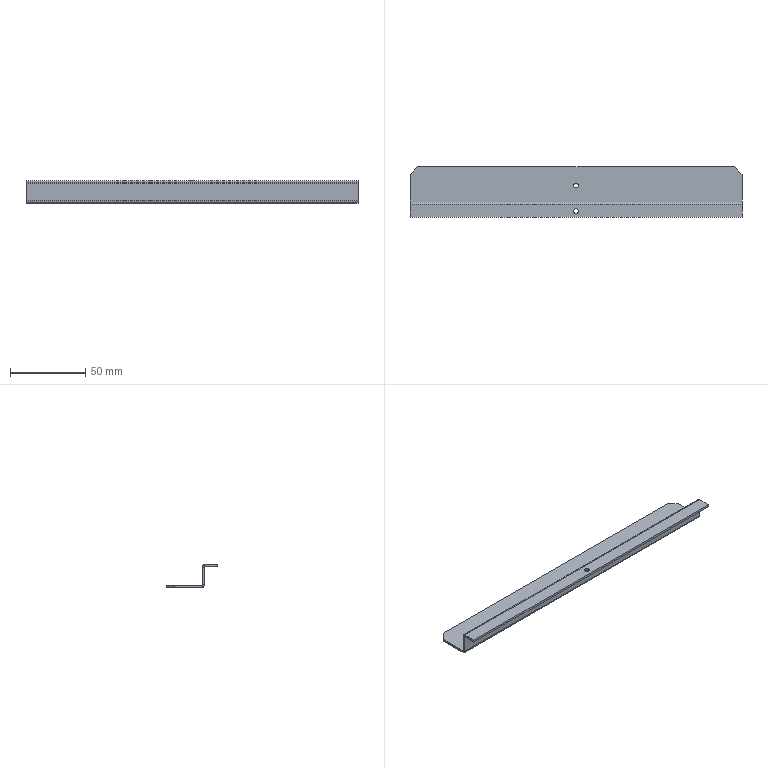Part | SolidWorks | features EdgeFlange 2, ICE 2, Chamfer 1, FlatPattern 1, SMBaseFlange 1, SheetMetal 1 | 1 solid | 28 faces | box 220 x 33.5 x 15 mm | volume 15208 mm3 | plane 20 | cylinder 8 | commonest cylinder face diameters 3.2 x6 0.2 x2
STEP:
#1=CARTESIAN_POINT('',(-1.6,-17.,13.5));
#2=VERTEX_POINT('',#1);
#3=CARTESIAN_POINT('',(1.6,-17.,13.5));
#4=VERTEX_POINT('',#3);
#5=CARTESIAN_POINT('',(0.,-17.,13.5));
#6=DIRECTION('',(0.,0.,1.));
#7=DIRECTION('',(1.,0.,0.));
#8=AXIS2_PLACEMENT_3D('',#5,#6,#7);
#9=CIRCLE('',#8,1.6);
#10=EDGE_CURVE('',#2,#4,#9,.T.);
#11=ORIENTED_EDGE('',*,*,#10,.T.);
#12=CARTESIAN_POINT('',(1.6,-17.,12.));
#13=VERTEX_POINT('',#12);
#14=CARTESIAN_POINT('',(1.6,-17.,22.));
#15=DIRECTION('',(0.,0.,-1.));
#16=VECTOR('',#15,1000.);
#17=LINE('',#14,#16);
#18=EDGE_CURVE('',#4,#13,#17,.T.);
#19=ORIENTED_EDGE('',*,*,#18,.T.);
#20=CARTESIAN_POINT('',(-1.6,-17.,12.));
#21=VERTEX_POINT('',#20);
#22=CARTESIAN_POINT('',(0.,-17.,12.));
#23=DIRECTION('',(0.,0.,-1.));
#24=DIRECTION('',(-1.,0.,0.));
#25=AXIS2_PLACEMENT_3D('',#22,#23,#24);
#26=CIRCLE('',#25,1.6);
#27=EDGE_CURVE('',#13,#21,#26,.T.);
#28=ORIENTED_EDGE('',*,*,#27,.T.);
#29=CARTESIAN_POINT('',(-1.6,-17.,22.));
#30=DIRECTION('',(0.,0.,-1.));
#31=VECTOR('',#30,1000.);
#32=LINE('',#29,#31);
#33=EDGE_CURVE('',#2,#21,#32,.T.);
#34=ORIENTED_EDGE('',*,*,#33,.F.);
#35=EDGE_LOOP('',(#11,#19,#28,#34));
#36=FACE_OUTER_BOUND('',#35,.T.);
#37=CARTESIAN_POINT('',(0.,-17.,22.));
#38=DIRECTION('',(0.,0.,-1.));
#39=DIRECTION('',(-1.,0.,0.));
#40=AXIS2_PLACEMENT_3D('',#37,#38,#39);
#41=CYLINDRICAL_SURFACE('',#40,1.6);
#42=ADVANCED_FACE('',(#36),#41,.F.);
#43=CARTESIAN_POINT('',(-1.6,0.,0.));
#44=VERTEX_POINT('',#43);
#45=CARTESIAN_POINT('',(1.6,0.,0.));
#46=VERTEX_POINT('',#45);
#47=CARTESIAN_POINT('',(0.,0.,0.));
#48=DIRECTION('',(0.,0.,1.));
#49=DIRECTION('',(1.,0.,0.));
#50=AXIS2_PLACEMENT_3D('',#47,#48,#49);
#51=CIRCLE('',#50,1.6);
#52=EDGE_CURVE('',#44,#46,#51,.T.);
#53=ORIENTED_EDGE('',*,*,#52,.T.);
#54=CARTESIAN_POINT('',(1.6,0.,-1.5));
#55=VERTEX_POINT('',#54);
#56=CARTESIAN_POINT('',(1.6,0.,8.5));
#57=DIRECTION('',(0.,0.,-1.));
#58=VECTOR('',#57,1000.);
#59=LINE('',#56,#58);
#60=EDGE_CURVE('',#46,#55,#59,.T.);
#61=ORIENTED_EDGE('',*,*,#60,.T.);
#62=CARTESIAN_POINT('',(-1.6,0.,-1.5));
#63=VERTEX_POINT('',#62);
#64=CARTESIAN_POINT('',(0.,0.,-1.5));
#65=DIRECTION('',(0.,0.,-1.));
#66=DIRECTION('',(-1.,0.,0.));
#67=AXIS2_PLACEMENT_3D('',#64,#65,#66);
#68=CIRCLE('',#67,1.6);
#69=EDGE_CURVE('',#55,#63,#68,.T.);
#70=ORIENTED_EDGE('',*,*,#69,.T.);
#71=CARTESIAN_POINT('',(-1.6,0.,8.5));
#72=DIRECTION('',(0.,0.,-1.));
#73=VECTOR('',#72,1000.);
#74=LINE('',#71,#73);
#75=EDGE_CURVE('',#44,#63,#74,.T.);
#76=ORIENTED_EDGE('',*,*,#75,.F.);
#77=EDGE_LOOP('',(#53,#61,#70,#76));
#78=FACE_OUTER_BOUND('',#77,.T.);
#79=CARTESIAN_POINT('',(0.,0.,8.5));
#80=DIRECTION('',(0.,0.,-1.));
#81=DIRECTION('',(-1.,0.,0.));
#82=AXIS2_PLACEMENT_3D('',#79,#80,#81);
#83=CYLINDRICAL_SURFACE('',#82,1.6);
#84=ADVANCED_FACE('',(#78),#83,.F.);
#85=CARTESIAN_POINT('',(110.,-12.5,11.9));
#86=VERTEX_POINT('',#85);
#87=CARTESIAN_POINT('',(110.,-11.,11.9));
#88=VERTEX_POINT('',#87);
#89=CARTESIAN_POINT('',(110.,-12.5,11.9));
#90=DIRECTION('',(0.,1.,0.));
#91=VECTOR('',#90,1000.);
#92=LINE('',#89,#91);
#93=EDGE_CURVE('',#86,#88,#92,.T.);
#94=ORIENTED_EDGE('',*,*,#93,.F.);
#95=CARTESIAN_POINT('',(110.,-12.5,0.1));
#96=VERTEX_POINT('',#95);
#97=CARTESIAN_POINT('',(110.,-12.5,0.));
#98=DIRECTION('',(0.,0.,1.));
#99=VECTOR('',#98,1000.);
#100=LINE('',#97,#99);
#101=EDGE_CURVE('',#96,#86,#100,.T.);
#102=ORIENTED_EDGE('',*,*,#101,.F.);
#103=CARTESIAN_POINT('',(110.,-11.,0.1));
#104=VERTEX_POINT('',#103);
#105=CARTESIAN_POINT('',(110.,-11.,0.1));
#106=DIRECTION('',(0.,-1.,0.));
#107=VECTOR('',#106,1000.);
#108=LINE('',#105,#107);
#109=EDGE_CURVE('',#104,#96,#108,.T.);
#110=ORIENTED_EDGE('',*,*,#109,.F.);
#111=CARTESIAN_POINT('',(110.,-11.,13.5));
#112=DIRECTION('',(0.,0.,1.));
#113=VECTOR('',#112,1000.);
#114=LINE('',#111,#113);
#115=EDGE_CURVE('',#104,#88,#114,.T.);
#116=ORIENTED_EDGE('',*,*,#115,.T.);
#117=EDGE_LOOP('',(#94,#102,#110,#116));
#118=FACE_OUTER_BOUND('',#117,.T.);
#119=CARTESIAN_POINT('',(110.,-12.5,13.5));
#120=DIRECTION('',(-1.,0.,0.));
#121=DIRECTION('',(0.,0.,1.));
#122=AXIS2_PLACEMENT_3D('',#119,#120,#121);
#123=PLANE('',#122);
#124=ADVANCED_FACE('',(#118),#123,.F.);
#125=CARTESIAN_POINT('',(-110.,-12.5,11.9));
#126=VERTEX_POINT('',#125);
#127=CARTESIAN_POINT('',(-110.,-11.,11.9));
#128=VERTEX_POINT('',#127);
#129=CARTESIAN_POINT('',(-110.,-12.5,11.9));
#130=DIRECTION('',(0.,1.,0.));
#131=VECTOR('',#130,1000.);
#132=LINE('',#129,#131);
#133=EDGE_CURVE('',#126,#128,#132,.T.);
#134=ORIENTED_EDGE('',*,*,#133,.T.);
#135=CARTESIAN_POINT('',(-110.,-11.,0.1));
#136=VERTEX_POINT('',#135);
#137=CARTESIAN_POINT('',(-110.,-11.,0.));
#138=DIRECTION('',(0.,0.,-1.));
#139=VECTOR('',#138,1000.);
#140=LINE('',#137,#139);
#141=EDGE_CURVE('',#128,#136,#140,.T.);
#142=ORIENTED_EDGE('',*,*,#141,.T.);
#143=CARTESIAN_POINT('',(-110.,-12.5,0.1));
#144=VERTEX_POINT('',#143);
#145=CARTESIAN_POINT('',(-110.,-12.5,0.1));
#146=DIRECTION('',(0.,-1.,0.));
#147=VECTOR('',#146,1000.);
#148=LINE('',#145,#147);
#149=EDGE_CURVE('',#136,#144,#148,.T.);
#150=ORIENTED_EDGE('',*,*,#149,.T.);
#151=CARTESIAN_POINT('',(-110.,-12.5,0.));
#152=DIRECTION('',(0.,0.,-1.));
#153=VECTOR('',#152,1000.);
#154=LINE('',#151,#153);
#155=EDGE_CURVE('',#126,#144,#154,.T.);
#156=ORIENTED_EDGE('',*,*,#155,.F.);
#157=EDGE_LOOP('',(#134,#142,#150,#156));
#158=FACE_OUTER_BOUND('',#157,.T.);
#159=CARTESIAN_POINT('',(-110.,-12.5,0.));
#160=DIRECTION('',(1.,0.,0.));
#161=DIRECTION('',(0.,0.,-1.));
#162=AXIS2_PLACEMENT_3D('',#159,#160,#161);
#163=PLANE('',#162);
#164=ADVANCED_FACE('',(#158),#163,.F.);
#165=CARTESIAN_POINT('',(-110.,-12.5,11.9));
#166=DIRECTION('',(1.,0.,0.));
#167=VECTOR('',#166,1000.);
#168=LINE('',#165,#167);
#169=EDGE_CURVE('',#126,#86,#168,.T.);
#170=ORIENTED_EDGE('',*,*,#169,.F.);
#171=ORIENTED_EDGE('',*,*,#155,.T.);
#172=CARTESIAN_POINT('',(-110.,-12.5,0.1));
#173=DIRECTION('',(-1.,0.,0.));
#174=VECTOR('',#173,1000.);
#175=LINE('',#172,#174);
#176=EDGE_CURVE('',#96,#144,#175,.T.);
#177=ORIENTED_EDGE('',*,*,#176,.F.);
#178=ORIENTED_EDGE('',*,*,#101,.T.);
#179=EDGE_LOOP('',(#170,#171,#177,#178));
#180=FACE_OUTER_BOUND('',#179,.T.);
#181=CARTESIAN_POINT('',(110.,-12.5,0.));
#182=DIRECTION('',(0.,1.,0.));
#183=DIRECTION('',(0.,0.,1.));
#184=AXIS2_PLACEMENT_3D('',#181,#182,#183);
#185=PLANE('',#184);
#186=ADVANCED_FACE('',(#180),#185,.F.);
#187=ORIENTED_EDGE('',*,*,#141,.F.);
#188=CARTESIAN_POINT('',(-110.,-11.,11.9));
#189=DIRECTION('',(1.,0.,0.));
#190=VECTOR('',#189,1000.);
#191=LINE('',#188,#190);
#192=EDGE_CURVE('',#128,#88,#191,.T.);
#193=ORIENTED_EDGE('',*,*,#192,.T.);
#194=ORIENTED_EDGE('',*,*,#115,.F.);
#195=CARTESIAN_POINT('',(-110.,-11.,0.1));
#196=DIRECTION('',(1.,0.,0.));
#197=VECTOR('',#196,1000.);
#198=LINE('',#195,#197);
#199=EDGE_CURVE('',#136,#104,#198,.T.);
#200=ORIENTED_EDGE('',*,*,#199,.F.);
#201=EDGE_LOOP('',(#187,#193,#194,#200));
#202=FACE_OUTER_BOUND('',#201,.T.);
#203=CARTESIAN_POINT('',(110.,-11.,0.));
#204=DIRECTION('',(0.,1.,0.));
#205=DIRECTION('',(0.,0.,1.));
#206=AXIS2_PLACEMENT_3D('',#203,#204,#205);
#207=PLANE('',#206);
#208=ADVANCED_FACE('',(#202),#207,.T.);
#209=CARTESIAN_POINT('',(110.,-10.9,-1.5));
#210=VERTEX_POINT('',#209);
#211=CARTESIAN_POINT('',(110.,7.5,-1.5));
#212=VERTEX_POINT('',#211);
#213=CARTESIAN_POINT('',(110.,12.5,-1.5));
#214=DIRECTION('',(0.,1.,0.));
#215=VECTOR('',#214,1000.);
#216=LINE('',#213,#215);
#217=EDGE_CURVE('',#210,#212,#216,.T.);
#218=ORIENTED_EDGE('',*,*,#217,.T.);
#219=CARTESIAN_POINT('',(110.,7.5,0.));
#220=VERTEX_POINT('',#219);
#221=CARTESIAN_POINT('',(110.,7.5,-1.5));
#222=DIRECTION('',(0.,0.,1.));
#223=VECTOR('',#222,1000.);
#224=LINE('',#221,#223);
#225=EDGE_CURVE('',#212,#220,#224,.T.);
#226=ORIENTED_EDGE('',*,*,#225,.T.);
#227=CARTESIAN_POINT('',(110.,-10.9,0.));
#228=VERTEX_POINT('',#227);
#229=CARTESIAN_POINT('',(110.,12.5,0.));
#230=DIRECTION('',(0.,1.,0.));
#231=VECTOR('',#230,1000.);
#232=LINE('',#229,#231);
#233=EDGE_CURVE('',#228,#220,#232,.T.);
#234=ORIENTED_EDGE('',*,*,#233,.F.);
#235=CARTESIAN_POINT('',(110.,-10.9,0.));
#236=DIRECTION('',(0.,0.,-1.));
#237=VECTOR('',#236,1000.);
#238=LINE('',#235,#237);
#239=EDGE_CURVE('',#228,#210,#238,.T.);
#240=ORIENTED_EDGE('',*,*,#239,.T.);
#241=EDGE_LOOP('',(#218,#226,#234,#240));
#242=FACE_OUTER_BOUND('',#241,.T.);
#243=CARTESIAN_POINT('',(110.,12.5,-1.5));
#244=DIRECTION('',(1.,0.,0.));
#245=DIRECTION('',(0.,0.,-1.));
#246=AXIS2_PLACEMENT_3D('',#243,#244,#245);
#247=PLANE('',#246);
#248=ADVANCED_FACE('',(#242),#247,.T.);
#249=CARTESIAN_POINT('',(0.,0.,-1.5));
#250=DIRECTION('',(0.,0.,-1.));
#251=DIRECTION('',(-1.,0.,0.));
#252=AXIS2_PLACEMENT_3D('',#249,#250,#251);
#253=CIRCLE('',#252,1.6);
#254=EDGE_CURVE('',#63,#55,#253,.T.);
#255=ORIENTED_EDGE('',*,*,#254,.F.);
#256=ORIENTED_EDGE('',*,*,#69,.F.);
#257=EDGE_LOOP('',(#255,#256));
#258=FACE_BOUND('',#257,.T.);
#259=CARTESIAN_POINT('',(105.,12.5,-1.5));
#260=VERTEX_POINT('',#259);
#261=CARTESIAN_POINT('',(-105.,12.5,-1.5));
#262=VERTEX_POINT('',#261);
#263=CARTESIAN_POINT('',(-110.,12.5,-1.5));
#264=DIRECTION('',(-1.,0.,0.));
#265=VECTOR('',#264,1000.);
#266=LINE('',#263,#265);
#267=EDGE_CURVE('',#260,#262,#266,.T.);
#268=ORIENTED_EDGE('',*,*,#267,.F.);
#269=CARTESIAN_POINT('',(110.,7.5,-1.5));
#270=DIRECTION('',(0.7071,-0.7071,0.));
#271=VECTOR('',#270,1000.);
#272=LINE('',#269,#271);
#273=EDGE_CURVE('',#260,#212,#272,.T.);
#274=ORIENTED_EDGE('',*,*,#273,.T.);
#275=ORIENTED_EDGE('',*,*,#217,.F.);
#276=CARTESIAN_POINT('',(-110.,-10.9,-1.5));
#277=VERTEX_POINT('',#276);
#278=CARTESIAN_POINT('',(110.,-10.9,-1.5));
#279=DIRECTION('',(-1.,0.,0.));
#280=VECTOR('',#279,1000.);
#281=LINE('',#278,#280);
#282=EDGE_CURVE('',#210,#277,#281,.T.);
#283=ORIENTED_EDGE('',*,*,#282,.T.);
#284=CARTESIAN_POINT('',(-110.,7.5,-1.5));
#285=VERTEX_POINT('',#284);
#286=CARTESIAN_POINT('',(-110.,12.5,-1.5));
#287=DIRECTION('',(0.,-1.,0.));
#288=VECTOR('',#287,1000.);
#289=LINE('',#286,#288);
#290=EDGE_CURVE('',#285,#277,#289,.T.);
#291=ORIENTED_EDGE('',*,*,#290,.F.);
#292=CARTESIAN_POINT('',(-105.,12.5,-1.5));
#293=DIRECTION('',(0.7071,0.7071,0.));
#294=VECTOR('',#293,1000.);
#295=LINE('',#292,#294);
#296=EDGE_CURVE('',#285,#262,#295,.T.);
#297=ORIENTED_EDGE('',*,*,#296,.T.);
#298=EDGE_LOOP('',(#268,#274,#275,#283,#291,#297));
#299=FACE_OUTER_BOUND('',#298,.T.);
#300=CARTESIAN_POINT('',(110.,-12.5,-1.5));
#301=DIRECTION('',(0.,0.,1.));
#302=DIRECTION('',(1.,0.,0.));
#303=AXIS2_PLACEMENT_3D('',#300,#301,#302);
#304=PLANE('',#303);
#305=ADVANCED_FACE('',(#258,#299),#304,.F.);
#306=ORIENTED_EDGE('',*,*,#52,.F.);
#307=CARTESIAN_POINT('',(0.,0.,0.));
#308=DIRECTION('',(0.,0.,1.));
#309=DIRECTION('',(1.,0.,0.));
#310=AXIS2_PLACEMENT_3D('',#307,#308,#309);
#311=CIRCLE('',#310,1.6);
#312=EDGE_CURVE('',#46,#44,#311,.T.);
#313=ORIENTED_EDGE('',*,*,#312,.F.);
#314=EDGE_LOOP('',(#306,#313));
#315=FACE_BOUND('',#314,.T.);
#316=ORIENTED_EDGE('',*,*,#233,.T.);
#317=CARTESIAN_POINT('',(105.,12.5,0.));
#318=VERTEX_POINT('',#317);
#319=CARTESIAN_POINT('',(120.,-2.5,0.));
#320=DIRECTION('',(-0.7071,0.7071,0.));
#321=VECTOR('',#320,1000.);
#322=LINE('',#319,#321);
#323=EDGE_CURVE('',#220,#318,#322,.T.);
#324=ORIENTED_EDGE('',*,*,#323,.T.);
#325=CARTESIAN_POINT('',(-105.,12.5,0.));
#326=VERTEX_POINT('',#325);
#327=CARTESIAN_POINT('',(-110.,12.5,0.));
#328=DIRECTION('',(-1.,0.,0.));
#329=VECTOR('',#328,1000.);
#330=LINE('',#327,#329);
#331=EDGE_CURVE('',#318,#326,#330,.T.);
#332=ORIENTED_EDGE('',*,*,#331,.T.);
#333=CARTESIAN_POINT('',(-110.,7.5,0.));
#334=VERTEX_POINT('',#333);
#335=CARTESIAN_POINT('',(-10.,107.5,0.));
#336=DIRECTION('',(-0.7071,-0.7071,0.));
#337=VECTOR('',#336,1000.);
#338=LINE('',#335,#337);
#339=EDGE_CURVE('',#326,#334,#338,.T.);
#340=ORIENTED_EDGE('',*,*,#339,.T.);
#341=CARTESIAN_POINT('',(-110.,-10.9,0.));
#342=VERTEX_POINT('',#341);
#343=CARTESIAN_POINT('',(-110.,12.5,0.));
#344=DIRECTION('',(0.,-1.,0.));
#345=VECTOR('',#344,1000.);
#346=LINE('',#343,#345);
#347=EDGE_CURVE('',#334,#342,#346,.T.);
#348=ORIENTED_EDGE('',*,*,#347,.T.);
#349=CARTESIAN_POINT('',(110.,-10.9,0.));
#350=DIRECTION('',(-1.,0.,0.));
#351=VECTOR('',#350,1000.);
#352=LINE('',#349,#351);
#353=EDGE_CURVE('',#228,#342,#352,.T.);
#354=ORIENTED_EDGE('',*,*,#353,.F.);
#355=EDGE_LOOP('',(#316,#324,#332,#340,#348,#354));
#356=FACE_OUTER_BOUND('',#355,.T.);
#357=CARTESIAN_POINT('',(110.,-12.5,0.));
#358=DIRECTION('',(0.,0.,1.));
#359=DIRECTION('',(1.,0.,0.));
#360=AXIS2_PLACEMENT_3D('',#357,#358,#359);
#361=PLANE('',#360);
#362=ADVANCED_FACE('',(#315,#356),#361,.T.);
#363=ORIENTED_EDGE('',*,*,#347,.F.);
#364=CARTESIAN_POINT('',(-110.,7.5,-1.5));
#365=DIRECTION('',(0.,0.,-1.));
#366=VECTOR('',#365,1000.);
#367=LINE('',#364,#366);
#368=EDGE_CURVE('',#334,#285,#367,.T.);
#369=ORIENTED_EDGE('',*,*,#368,.T.);
#370=ORIENTED_EDGE('',*,*,#290,.T.);
#371=CARTESIAN_POINT('',(-110.,-10.9,0.));
#372=DIRECTION('',(0.,0.,-1.));
#373=VECTOR('',#372,1000.);
#374=LINE('',#371,#373);
#375=EDGE_CURVE('',#342,#277,#374,.T.);
#376=ORIENTED_EDGE('',*,*,#375,.F.);
#377=EDGE_LOOP('',(#363,#369,#370,#376));
#378=FACE_OUTER_BOUND('',#377,.T.);
#379=CARTESIAN_POINT('',(-110.,12.5,-1.5));
#380=DIRECTION('',(-1.,0.,0.));
#381=DIRECTION('',(0.,0.,1.));
#382=AXIS2_PLACEMENT_3D('',#379,#380,#381);
#383=PLANE('',#382);
#384=ADVANCED_FACE('',(#378),#383,.T.);
#385=ORIENTED_EDGE('',*,*,#331,.F.);
#386=CARTESIAN_POINT('',(105.,12.5,-1.5));
#387=DIRECTION('',(0.,0.,-1.));
#388=VECTOR('',#387,1000.);
#389=LINE('',#386,#388);
#390=EDGE_CURVE('',#318,#260,#389,.T.);
#391=ORIENTED_EDGE('',*,*,#390,.T.);
#392=ORIENTED_EDGE('',*,*,#267,.T.);
#393=CARTESIAN_POINT('',(-105.,12.5,-1.5));
#394=DIRECTION('',(0.,0.,1.));
#395=VECTOR('',#394,1000.);
#396=LINE('',#393,#395);
#397=EDGE_CURVE('',#262,#326,#396,.T.);
#398=ORIENTED_EDGE('',*,*,#397,.T.);
#399=EDGE_LOOP('',(#385,#391,#392,#398));
#400=FACE_OUTER_BOUND('',#399,.T.);
#401=CARTESIAN_POINT('',(-110.,12.5,-1.5));
#402=DIRECTION('',(0.,1.,0.));
#403=DIRECTION('',(0.,0.,1.));
#404=AXIS2_PLACEMENT_3D('',#401,#402,#403);
#405=PLANE('',#404);
#406=ADVANCED_FACE('',(#400),#405,.T.);
#407=ORIENTED_EDGE('',*,*,#149,.F.);
#408=CARTESIAN_POINT('',(-110.,-10.9,0.1));
#409=DIRECTION('',(-1.,0.,0.));
#410=DIRECTION('',(0.,0.,-1.));
#411=AXIS2_PLACEMENT_3D('',#408,#409,#410);
#412=CIRCLE('',#411,0.1);
#413=EDGE_CURVE('',#342,#136,#412,.T.);
#414=ORIENTED_EDGE('',*,*,#413,.F.);
#415=ORIENTED_EDGE('',*,*,#375,.T.);
#416=CARTESIAN_POINT('',(-110.,-10.9,0.1));
#417=DIRECTION('',(-1.,0.,0.));
#418=DIRECTION('',(0.,0.,-1.));
#419=AXIS2_PLACEMENT_3D('',#416,#417,#418);
#420=CIRCLE('',#419,1.6);
#421=EDGE_CURVE('',#277,#144,#420,.T.);
#422=ORIENTED_EDGE('',*,*,#421,.T.);
#423=EDGE_LOOP('',(#407,#414,#415,#422));
#424=FACE_OUTER_BOUND('',#423,.T.);
#425=CARTESIAN_POINT('',(-110.,-10.9,0.1));
#426=DIRECTION('',(-1.,0.,0.));
#427=DIRECTION('',(0.,0.,1.));
#428=AXIS2_PLACEMENT_3D('',#425,#426,#427);
#429=PLANE('',#428);
#430=ADVANCED_FACE('',(#424),#429,.T.);
#431=CARTESIAN_POINT('',(110.,-10.9,0.1));
#432=DIRECTION('',(1.,0.,0.));
#433=DIRECTION('',(0.,0.,-1.));
#434=AXIS2_PLACEMENT_3D('',#431,#432,#433);
#435=CIRCLE('',#434,0.1);
#436=EDGE_CURVE('',#104,#228,#435,.T.);
#437=ORIENTED_EDGE('',*,*,#436,.F.);
#438=ORIENTED_EDGE('',*,*,#109,.T.);
#439=CARTESIAN_POINT('',(110.,-10.9,0.1));
#440=DIRECTION('',(1.,0.,0.));
#441=DIRECTION('',(0.,0.,-1.));
#442=AXIS2_PLACEMENT_3D('',#439,#440,#441);
#443=CIRCLE('',#442,1.6);
#444=EDGE_CURVE('',#96,#210,#443,.T.);
#445=ORIENTED_EDGE('',*,*,#444,.T.);
#446=ORIENTED_EDGE('',*,*,#239,.F.);
#447=EDGE_LOOP('',(#437,#438,#445,#446));
#448=FACE_OUTER_BOUND('',#447,.T.);
#449=CARTESIAN_POINT('',(110.,-10.9,0.1));
#450=DIRECTION('',(-1.,0.,0.));
#451=DIRECTION('',(0.,0.,1.));
#452=AXIS2_PLACEMENT_3D('',#449,#450,#451);
#453=PLANE('',#452);
#454=ADVANCED_FACE('',(#448),#453,.F.);
#455=ORIENTED_EDGE('',*,*,#282,.F.);
#456=ORIENTED_EDGE('',*,*,#444,.F.);
#457=ORIENTED_EDGE('',*,*,#176,.T.);
#458=ORIENTED_EDGE('',*,*,#421,.F.);
#459=EDGE_LOOP('',(#455,#456,#457,#458));
#460=FACE_OUTER_BOUND('',#459,.T.);
#461=CARTESIAN_POINT('',(110.,-10.9,0.1));
#462=DIRECTION('',(1.,0.,0.));
#463=DIRECTION('',(0.,-1.,0.));
#464=AXIS2_PLACEMENT_3D('',#461,#462,#463);
#465=CYLINDRICAL_SURFACE('',#464,1.6);
#466=ADVANCED_FACE('',(#460),#465,.T.);
#467=ORIENTED_EDGE('',*,*,#353,.T.);
#468=ORIENTED_EDGE('',*,*,#413,.T.);
#469=ORIENTED_EDGE('',*,*,#199,.T.);
#470=ORIENTED_EDGE('',*,*,#436,.T.);
#471=EDGE_LOOP('',(#467,#468,#469,#470));
#472=FACE_OUTER_BOUND('',#471,.T.);
#473=CARTESIAN_POINT('',(110.,-10.9,0.1));
#474=DIRECTION('',(1.,0.,0.));
#475=DIRECTION('',(0.,-1.,0.));
#476=AXIS2_PLACEMENT_3D('',#473,#474,#475);
#477=CYLINDRICAL_SURFACE('',#476,0.1);
#478=ADVANCED_FACE('',(#472),#477,.F.);
#479=CARTESIAN_POINT('',(110.,-12.6,12.));
#480=VERTEX_POINT('',#479);
#481=CARTESIAN_POINT('',(110.,-12.6,13.5));
#482=VERTEX_POINT('',#481);
#483=CARTESIAN_POINT('',(110.,-12.6,13.5));
#484=DIRECTION('',(0.,0.,1.));
#485=VECTOR('',#484,1000.);
#486=LINE('',#483,#485);
#487=EDGE_CURVE('',#480,#482,#486,.T.);
#488=ORIENTED_EDGE('',*,*,#487,.F.);
#489=CARTESIAN_POINT('',(110.,-12.6,11.9));
#490=DIRECTION('',(1.,0.,0.));
#491=DIRECTION('',(0.,0.,1.));
#492=AXIS2_PLACEMENT_3D('',#489,#490,#491);
#493=CIRCLE('',#492,0.1);
#494=EDGE_CURVE('',#86,#480,#493,.T.);
#495=ORIENTED_EDGE('',*,*,#494,.F.);
#496=ORIENTED_EDGE('',*,*,#93,.T.);
#497=CARTESIAN_POINT('',(110.,-12.6,11.9));
#498=DIRECTION('',(1.,0.,0.));
#499=DIRECTION('',(0.,0.,1.));
#500=AXIS2_PLACEMENT_3D('',#497,#498,#499);
#501=CIRCLE('',#500,1.6);
#502=EDGE_CURVE('',#88,#482,#501,.T.);
#503=ORIENTED_EDGE('',*,*,#502,.T.);
#504=EDGE_LOOP('',(#488,#495,#496,#503));
#505=FACE_OUTER_BOUND('',#504,.T.);
#506=CARTESIAN_POINT('',(110.,-12.6,11.9));
#507=DIRECTION('',(1.,0.,0.));
#508=DIRECTION('',(0.,0.,-1.));
#509=AXIS2_PLACEMENT_3D('',#506,#507,#508);
#510=PLANE('',#509);
#511=ADVANCED_FACE('',(#505),#510,.T.);
#512=CARTESIAN_POINT('',(-110.,-12.6,12.));
#513=VERTEX_POINT('',#512);
#514=CARTESIAN_POINT('',(-110.,-12.6,11.9));
#515=DIRECTION('',(-1.,0.,0.));
#516=DIRECTION('',(0.,0.,1.));
#517=AXIS2_PLACEMENT_3D('',#514,#515,#516);
#518=CIRCLE('',#517,0.1);
#519=EDGE_CURVE('',#513,#126,#518,.T.);
#520=ORIENTED_EDGE('',*,*,#519,.F.);
#521=CARTESIAN_POINT('',(-110.,-12.6,13.5));
#522=VERTEX_POINT('',#521);
#523=CARTESIAN_POINT('',(-110.,-12.6,12.));
#524=DIRECTION('',(0.,0.,1.));
#525=VECTOR('',#524,1000.);
#526=LINE('',#523,#525);
#527=EDGE_CURVE('',#513,#522,#526,.T.);
#528=ORIENTED_EDGE('',*,*,#527,.T.);
#529=CARTESIAN_POINT('',(-110.,-12.6,11.9));
#530=DIRECTION('',(-1.,0.,0.));
#531=DIRECTION('',(0.,0.,1.));
#532=AXIS2_PLACEMENT_3D('',#529,#530,#531);
#533=CIRCLE('',#532,1.6);
#534=EDGE_CURVE('',#522,#128,#533,.T.);
#535=ORIENTED_EDGE('',*,*,#534,.T.);
#536=ORIENTED_EDGE('',*,*,#133,.F.);
#537=EDGE_LOOP('',(#520,#528,#535,#536));
#538=FACE_OUTER_BOUND('',#537,.T.);
#539=CARTESIAN_POINT('',(-110.,-12.6,11.9));
#540=DIRECTION('',(1.,0.,0.));
#541=DIRECTION('',(0.,0.,-1.));
#542=AXIS2_PLACEMENT_3D('',#539,#540,#541);
#543=PLANE('',#542);
#544=ADVANCED_FACE('',(#538),#543,.F.);
#545=ORIENTED_EDGE('',*,*,#192,.F.);
#546=ORIENTED_EDGE('',*,*,#534,.F.);
#547=CARTESIAN_POINT('',(-110.,-12.6,13.5));
#548=DIRECTION('',(-1.,0.,0.));
#549=VECTOR('',#548,1000.);
#550=LINE('',#547,#549);
#551=EDGE_CURVE('',#482,#522,#550,.T.);
#552=ORIENTED_EDGE('',*,*,#551,.F.);
#553=ORIENTED_EDGE('',*,*,#502,.F.);
#554=EDGE_LOOP('',(#545,#546,#552,#553));
#555=FACE_OUTER_BOUND('',#554,.T.);
#556=CARTESIAN_POINT('',(-110.,-12.6,11.9));
#557=DIRECTION('',(-1.,0.,0.));
#558=DIRECTION('',(0.,0.,1.));
#559=AXIS2_PLACEMENT_3D('',#556,#557,#558);
#560=CYLINDRICAL_SURFACE('',#559,1.6);
#561=ADVANCED_FACE('',(#555),#560,.T.);
#562=ORIENTED_EDGE('',*,*,#169,.T.);
#563=ORIENTED_EDGE('',*,*,#494,.T.);
#564=CARTESIAN_POINT('',(110.,-12.6,12.));
#565=DIRECTION('',(-1.,0.,0.));
#566=VECTOR('',#565,1000.);
#567=LINE('',#564,#566);
#568=EDGE_CURVE('',#480,#513,#567,.T.);
#569=ORIENTED_EDGE('',*,*,#568,.T.);
#570=ORIENTED_EDGE('',*,*,#519,.T.);
#571=EDGE_LOOP('',(#562,#563,#569,#570));
#572=FACE_OUTER_BOUND('',#571,.T.);
#573=CARTESIAN_POINT('',(-110.,-12.6,11.9));
#574=DIRECTION('',(-1.,0.,0.));
#575=DIRECTION('',(0.,0.,1.));
#576=AXIS2_PLACEMENT_3D('',#573,#574,#575);
#577=CYLINDRICAL_SURFACE('',#576,0.1);
#578=ADVANCED_FACE('',(#572),#577,.F.);
#579=CARTESIAN_POINT('',(-110.,-21.,13.5));
#580=VERTEX_POINT('',#579);
#581=CARTESIAN_POINT('',(-110.,-12.5,13.5));
#582=DIRECTION('',(0.,1.,0.));
#583=VECTOR('',#582,1000.);
#584=LINE('',#581,#583);
#585=EDGE_CURVE('',#580,#522,#584,.T.);
#586=ORIENTED_EDGE('',*,*,#585,.T.);
#587=ORIENTED_EDGE('',*,*,#527,.F.);
#588=CARTESIAN_POINT('',(-110.,-21.,12.));
#589=VERTEX_POINT('',#588);
#590=CARTESIAN_POINT('',(-110.,-12.5,12.));
#591=DIRECTION('',(0.,1.,0.));
#592=VECTOR('',#591,1000.);
#593=LINE('',#590,#592);
#594=EDGE_CURVE('',#589,#513,#593,.T.);
#595=ORIENTED_EDGE('',*,*,#594,.F.);
#596=CARTESIAN_POINT('',(-110.,-21.,13.5));
#597=DIRECTION('',(0.,0.,-1.));
#598=VECTOR('',#597,1000.);
#599=LINE('',#596,#598);
#600=EDGE_CURVE('',#580,#589,#599,.T.);
#601=ORIENTED_EDGE('',*,*,#600,.F.);
#602=EDGE_LOOP('',(#586,#587,#595,#601));
#603=FACE_OUTER_BOUND('',#602,.T.);
#604=CARTESIAN_POINT('',(-110.,-12.5,13.5));
#605=DIRECTION('',(-1.,0.,0.));
#606=DIRECTION('',(0.,0.,1.));
#607=AXIS2_PLACEMENT_3D('',#604,#605,#606);
#608=PLANE('',#607);
#609=ADVANCED_FACE('',(#603),#608,.T.);
#610=CARTESIAN_POINT('',(110.,-21.,12.));
#611=VERTEX_POINT('',#610);
#612=CARTESIAN_POINT('',(110.,-12.5,12.));
#613=DIRECTION('',(0.,-1.,0.));
#614=VECTOR('',#613,1000.);
#615=LINE('',#612,#614);
#616=EDGE_CURVE('',#480,#611,#615,.T.);
#617=ORIENTED_EDGE('',*,*,#616,.F.);
#618=ORIENTED_EDGE('',*,*,#487,.T.);
#619=CARTESIAN_POINT('',(110.,-21.,13.5));
#620=VERTEX_POINT('',#619);
#621=CARTESIAN_POINT('',(110.,-21.,13.5));
#622=DIRECTION('',(0.,-1.,0.));
#623=VECTOR('',#622,1000.);
#624=LINE('',#621,#623);
#625=EDGE_CURVE('',#482,#620,#624,.T.);
#626=ORIENTED_EDGE('',*,*,#625,.T.);
#627=CARTESIAN_POINT('',(110.,-21.,13.5));
#628=DIRECTION('',(0.,0.,-1.));
#629=VECTOR('',#628,1000.);
#630=LINE('',#627,#629);
#631=EDGE_CURVE('',#620,#611,#630,.T.);
#632=ORIENTED_EDGE('',*,*,#631,.T.);
#633=EDGE_LOOP('',(#617,#618,#626,#632));
#634=FACE_OUTER_BOUND('',#633,.T.);
#635=CARTESIAN_POINT('',(110.,-21.,13.5));
#636=DIRECTION('',(1.,0.,0.));
#637=DIRECTION('',(0.,0.,-1.));
#638=AXIS2_PLACEMENT_3D('',#635,#636,#637);
#639=PLANE('',#638);
#640=ADVANCED_FACE('',(#634),#639,.T.);
#641=ORIENTED_EDGE('',*,*,#10,.F.);
#642=CARTESIAN_POINT('',(0.,-17.,13.5));
#643=DIRECTION('',(0.,0.,1.));
#644=DIRECTION('',(1.,0.,0.));
#645=AXIS2_PLACEMENT_3D('',#642,#643,#644);
#646=CIRCLE('',#645,1.6);
#647=EDGE_CURVE('',#4,#2,#646,.T.);
#648=ORIENTED_EDGE('',*,*,#647,.F.);
#649=EDGE_LOOP('',(#641,#648));
#650=FACE_BOUND('',#649,.T.);
#651=ORIENTED_EDGE('',*,*,#625,.F.);
#652=ORIENTED_EDGE('',*,*,#551,.T.);
#653=ORIENTED_EDGE('',*,*,#585,.F.);
#654=CARTESIAN_POINT('',(-110.,-21.,13.5));
#655=DIRECTION('',(-1.,0.,0.));
#656=VECTOR('',#655,1000.);
#657=LINE('',#654,#656);
#658=EDGE_CURVE('',#620,#580,#657,.T.);
#659=ORIENTED_EDGE('',*,*,#658,.F.);
#660=EDGE_LOOP('',(#651,#652,#653,#659));
#661=FACE_OUTER_BOUND('',#660,.T.);
#662=CARTESIAN_POINT('',(-110.,-12.5,13.5));
#663=DIRECTION('',(0.,0.,1.));
#664=DIRECTION('',(1.,0.,0.));
#665=AXIS2_PLACEMENT_3D('',#662,#663,#664);
#666=PLANE('',#665);
#667=ADVANCED_FACE('',(#650,#661),#666,.T.);
#668=CARTESIAN_POINT('',(0.,-17.,12.));
#669=DIRECTION('',(0.,0.,-1.));
#670=DIRECTION('',(-1.,0.,0.));
#671=AXIS2_PLACEMENT_3D('',#668,#669,#670);
#672=CIRCLE('',#671,1.6);
#673=EDGE_CURVE('',#21,#13,#672,.T.);
#674=ORIENTED_EDGE('',*,*,#673,.F.);
#675=ORIENTED_EDGE('',*,*,#27,.F.);
#676=EDGE_LOOP('',(#674,#675));
#677=FACE_BOUND('',#676,.T.);
#678=ORIENTED_EDGE('',*,*,#568,.F.);
#679=ORIENTED_EDGE('',*,*,#616,.T.);
#680=CARTESIAN_POINT('',(-110.,-21.,12.));
#681=DIRECTION('',(-1.,0.,0.));
#682=VECTOR('',#681,1000.);
#683=LINE('',#680,#682);
#684=EDGE_CURVE('',#611,#589,#683,.T.);
#685=ORIENTED_EDGE('',*,*,#684,.T.);
#686=ORIENTED_EDGE('',*,*,#594,.T.);
#687=EDGE_LOOP('',(#678,#679,#685,#686));
#688=FACE_OUTER_BOUND('',#687,.T.);
#689=CARTESIAN_POINT('',(-110.,-12.5,12.));
#690=DIRECTION('',(0.,0.,1.));
#691=DIRECTION('',(1.,0.,0.));
#692=AXIS2_PLACEMENT_3D('',#689,#690,#691);
#693=PLANE('',#692);
#694=ADVANCED_FACE('',(#677,#688),#693,.F.);
#695=ORIENTED_EDGE('',*,*,#684,.F.);
#696=ORIENTED_EDGE('',*,*,#631,.F.);
#697=ORIENTED_EDGE('',*,*,#658,.T.);
#698=ORIENTED_EDGE('',*,*,#600,.T.);
#699=EDGE_LOOP('',(#695,#696,#697,#698));
#700=FACE_OUTER_BOUND('',#699,.T.);
#701=CARTESIAN_POINT('',(-110.,-21.,13.5));
#702=DIRECTION('',(0.,-1.,0.));
#703=DIRECTION('',(0.,0.,-1.));
#704=AXIS2_PLACEMENT_3D('',#701,#702,#703);
#705=PLANE('',#704);
#706=ADVANCED_FACE('',(#700),#705,.T.);
#707=ORIENTED_EDGE('',*,*,#60,.F.);
#708=ORIENTED_EDGE('',*,*,#312,.T.);
#709=ORIENTED_EDGE('',*,*,#75,.T.);
#710=ORIENTED_EDGE('',*,*,#254,.T.);
#711=EDGE_LOOP('',(#707,#708,#709,#710));
#712=FACE_OUTER_BOUND('',#711,.T.);
#713=CARTESIAN_POINT('',(0.,0.,8.5));
#714=DIRECTION('',(0.,0.,-1.));
#715=DIRECTION('',(-1.,0.,0.));
#716=AXIS2_PLACEMENT_3D('',#713,#714,#715);
#717=CYLINDRICAL_SURFACE('',#716,1.6);
#718=ADVANCED_FACE('',(#712),#717,.F.);
#719=ORIENTED_EDGE('',*,*,#18,.F.);
#720=ORIENTED_EDGE('',*,*,#647,.T.);
#721=ORIENTED_EDGE('',*,*,#33,.T.);
#722=ORIENTED_EDGE('',*,*,#673,.T.);
#723=EDGE_LOOP('',(#719,#720,#721,#722));
#724=FACE_OUTER_BOUND('',#723,.T.);
#725=CARTESIAN_POINT('',(0.,-17.,22.));
#726=DIRECTION('',(0.,0.,-1.));
#727=DIRECTION('',(-1.,0.,0.));
#728=AXIS2_PLACEMENT_3D('',#725,#726,#727);
#729=CYLINDRICAL_SURFACE('',#728,1.6);
#730=ADVANCED_FACE('',(#724),#729,.F.);
#731=ORIENTED_EDGE('',*,*,#273,.F.);
#732=ORIENTED_EDGE('',*,*,#390,.F.);
#733=ORIENTED_EDGE('',*,*,#323,.F.);
#734=ORIENTED_EDGE('',*,*,#225,.F.);
#735=EDGE_LOOP('',(#731,#732,#733,#734));
#736=FACE_OUTER_BOUND('',#735,.T.);
#737=CARTESIAN_POINT('',(110.,7.5,-1.5));
#738=DIRECTION('',(-0.7071,-0.7071,0.));
#739=DIRECTION('',(0.7071,-0.7071,0.));
#740=AXIS2_PLACEMENT_3D('',#737,#738,#739);
#741=PLANE('',#740);
#742=ADVANCED_FACE('',(#736),#741,.F.);
#743=ORIENTED_EDGE('',*,*,#296,.F.);
#744=ORIENTED_EDGE('',*,*,#368,.F.);
#745=ORIENTED_EDGE('',*,*,#339,.F.);
#746=ORIENTED_EDGE('',*,*,#397,.F.);
#747=EDGE_LOOP('',(#743,#744,#745,#746));
#748=FACE_OUTER_BOUND('',#747,.T.);
#749=CARTESIAN_POINT('',(-105.,12.5,-1.5));
#750=DIRECTION('',(0.7071,-0.7071,0.));
#751=DIRECTION('',(0.7071,0.7071,0.));
#752=AXIS2_PLACEMENT_3D('',#749,#750,#751);
#753=PLANE('',#752);
#754=ADVANCED_FACE('',(#748),#753,.F.);
#755=CLOSED_SHELL('',(#42,#84,#124,#164,#186,#208,#248,#305,#362,#384,#406,#430,#454,#466,#478,#511,#544,#561,#578,#609,#640,#667,#694,#706,#718,#730,#742,#754));
#756=MANIFOLD_SOLID_BREP('',#755);
#757=CARTESIAN_POINT('',(0.,0.,0.));
#758=DIRECTION('',(0.,0.,1.));
#759=DIRECTION('',(1.,0.,0.));
#760=AXIS2_PLACEMENT_3D('',#757,#758,#759);
#761=(LENGTH_UNIT()NAMED_UNIT(*)SI_UNIT(.MILLI.,.METRE.));
#762=UNCERTAINTY_MEASURE_WITH_UNIT(LENGTH_MEASURE(0.00001),#761,'','');
#763=(NAMED_UNIT(*)PLANE_ANGLE_UNIT()SI_UNIT($,.RADIAN.));
#764=(NAMED_UNIT(*)SI_UNIT($,.STERADIAN.)SOLID_ANGLE_UNIT());
#765=(GEOMETRIC_REPRESENTATION_CONTEXT(3)GLOBAL_UNCERTAINTY_ASSIGNED_CONTEXT((#762))GLOBAL_UNIT_ASSIGNED_CONTEXT((#761,#763,#764))REPRESENTATION_CONTEXT('',''));
#766=ADVANCED_BREP_SHAPE_REPRESENTATION('',(#756,#760),#765);